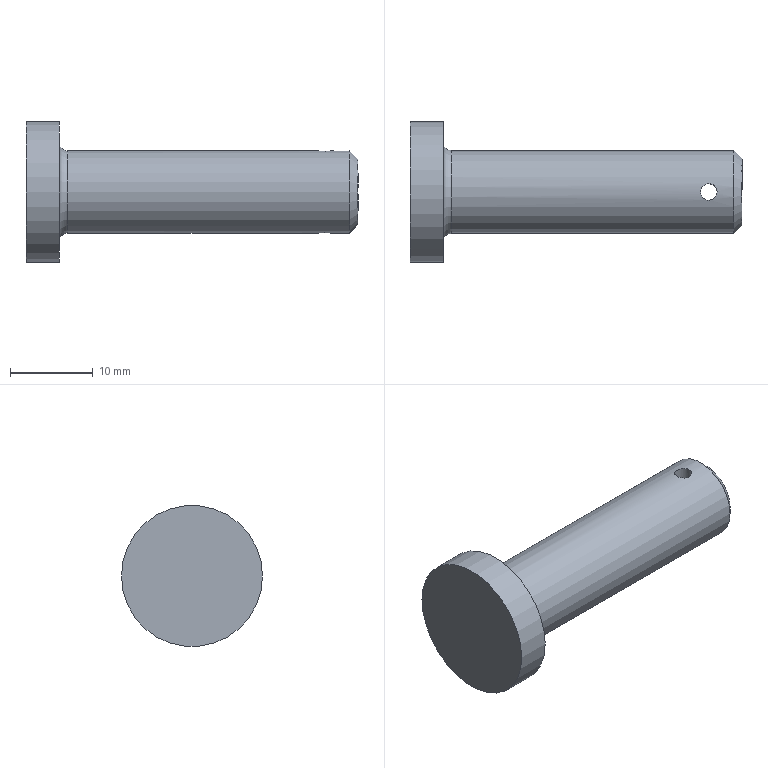Part | NX | features DATUM_CSYS 3, SKETCH 2, EXTRUDE 1, SWP104 1 | 1 solid | 8 faces | box 40 x 17 x 17 mm | volume 3696 mm3 | cylinder 3 | plane 3 | torus 1 | cone 1 | commonest cylinder face diameters 2 x1 10 x1 17 x1
STEP:
#1=CARTESIAN_POINT('',(39.,5.,0.));
#2=VERTEX_POINT('',#1);
#3=CARTESIAN_POINT('',(39.,0.,0.));
#4=DIRECTION('',(1.,0.,0.));
#5=DIRECTION('',(0.,1.,0.));
#6=AXIS2_PLACEMENT_3D('',#3,#4,#5);
#7=CIRCLE('',#6,5.);
#8=EDGE_CURVE('',#2,#2,#7,.T.);
#9=ORIENTED_EDGE('',*,*,#8,.F.);
#10=EDGE_LOOP('',(#9));
#11=FACE_BOUND('',#10,.T.);
#12=CARTESIAN_POINT('',(5.,5.,0.));
#13=VERTEX_POINT('',#12);
#14=CARTESIAN_POINT('',(5.,0.,0.));
#15=DIRECTION('',(1.,0.,0.));
#16=DIRECTION('',(0.,1.,0.));
#17=AXIS2_PLACEMENT_3D('',#14,#15,#16);
#18=CIRCLE('',#17,5.);
#19=EDGE_CURVE('',#13,#13,#18,.T.);
#20=ORIENTED_EDGE('',*,*,#19,.T.);
#21=EDGE_LOOP('',(#20));
#22=FACE_BOUND('',#21,.T.);
#23=CARTESIAN_POINT('',(35.,0.,-5.));
#24=VERTEX_POINT('',#23);
#25=CARTESIAN_POINT('',(35.217,-0.7844,-4.95));
#26=CARTESIAN_POINT('',(34.892,0.0001751,-5.025));
#27=CARTESIAN_POINT('',(35.217,0.7837,-4.95));
#28=CARTESIAN_POINT('',(35.999,1.108,-4.873));
#29=CARTESIAN_POINT('',(36.784,0.7838,-4.95));
#30=CARTESIAN_POINT('',(37.108,0.0003593,-5.025));
#31=CARTESIAN_POINT('',(36.784,-0.7828,-4.95));
#32=CARTESIAN_POINT('',(36.001,-1.108,-4.873));
#33=CARTESIAN_POINT('',(35.217,-0.7844,-4.95));
#34=CARTESIAN_POINT('',(34.892,0.0001751,-5.025));
#35=CARTESIAN_POINT('',(35.217,0.7837,-4.95));
#36=B_SPLINE_CURVE_WITH_KNOTS('',3,(#25,#26,#27,#28,#29,#30,#31,#32,#33,#34,#35),.UNSPECIFIED.,.T.,.F.,(1,1,1,1,1,1,1,1,1,1,1,1,1,1,1),(-0.00235,-0.001567,-0.0007835,0.,0.0007835,0.001567,0.00235,0.003134,0.003917,0.004701,0.005484,0.006268,0.007051,0.007835,0.008618),.UNSPECIFIED.);
#37=EDGE_CURVE('',#24,#24,#36,.T.);
#38=ORIENTED_EDGE('',*,*,#37,.F.);
#39=EDGE_LOOP('',(#38));
#40=FACE_BOUND('',#39,.T.);
#41=CARTESIAN_POINT('',(35.,0.,5.));
#42=VERTEX_POINT('',#41);
#43=CARTESIAN_POINT('',(35.217,0.7844,4.95));
#44=CARTESIAN_POINT('',(34.892,-0.0001751,5.025));
#45=CARTESIAN_POINT('',(35.217,-0.7837,4.95));
#46=CARTESIAN_POINT('',(35.999,-1.108,4.873));
#47=CARTESIAN_POINT('',(36.784,-0.7838,4.95));
#48=CARTESIAN_POINT('',(37.108,-0.0003593,5.025));
#49=CARTESIAN_POINT('',(36.784,0.7828,4.95));
#50=CARTESIAN_POINT('',(36.001,1.108,4.873));
#51=CARTESIAN_POINT('',(35.217,0.7844,4.95));
#52=CARTESIAN_POINT('',(34.892,-0.0001751,5.025));
#53=CARTESIAN_POINT('',(35.217,-0.7837,4.95));
#54=B_SPLINE_CURVE_WITH_KNOTS('',3,(#43,#44,#45,#46,#47,#48,#49,#50,#51,#52,#53),.UNSPECIFIED.,.T.,.F.,(1,1,1,1,1,1,1,1,1,1,1,1,1,1,1),(-0.00235,-0.001567,-0.0007835,0.,0.0007835,0.001567,0.00235,0.003134,0.003917,0.004701,0.005484,0.006268,0.007051,0.007835,0.008618),.UNSPECIFIED.);
#55=EDGE_CURVE('',#42,#42,#54,.T.);
#56=ORIENTED_EDGE('',*,*,#55,.F.);
#57=EDGE_LOOP('',(#56));
#58=FACE_BOUND('',#57,.T.);
#59=CARTESIAN_POINT('',(0.,0.,0.));
#60=DIRECTION('',(1.,0.,0.));
#61=DIRECTION('',(0.,1.,0.));
#62=AXIS2_PLACEMENT_3D('',#59,#60,#61);
#63=CYLINDRICAL_SURFACE('',#62,5.);
#64=ADVANCED_FACE('',(#11,#22,#40,#58),#63,.T.);
#65=CARTESIAN_POINT('',(0.,8.5,0.));
#66=VERTEX_POINT('',#65);
#67=CARTESIAN_POINT('',(0.,0.,0.));
#68=DIRECTION('',(1.,0.,0.));
#69=DIRECTION('',(0.,1.,0.));
#70=AXIS2_PLACEMENT_3D('',#67,#68,#69);
#71=CIRCLE('',#70,8.5);
#72=EDGE_CURVE('',#66,#66,#71,.T.);
#73=ORIENTED_EDGE('',*,*,#72,.F.);
#74=EDGE_LOOP('',(#73));
#75=FACE_BOUND('',#74,.T.);
#76=CARTESIAN_POINT('',(0.,0.,0.));
#77=DIRECTION('',(1.,0.,0.));
#78=DIRECTION('',(0.,1.,0.));
#79=AXIS2_PLACEMENT_3D('',#76,#77,#78);
#80=PLANE('',#79);
#81=ADVANCED_FACE('',(#75),#80,.F.);
#82=CARTESIAN_POINT('',(4.,8.5,0.));
#83=VERTEX_POINT('',#82);
#84=CARTESIAN_POINT('',(4.,0.,0.));
#85=DIRECTION('',(1.,0.,0.));
#86=DIRECTION('',(0.,1.,0.));
#87=AXIS2_PLACEMENT_3D('',#84,#85,#86);
#88=CIRCLE('',#87,8.5);
#89=EDGE_CURVE('',#83,#83,#88,.T.);
#90=ORIENTED_EDGE('',*,*,#89,.F.);
#91=EDGE_LOOP('',(#90));
#92=FACE_BOUND('',#91,.T.);
#93=ORIENTED_EDGE('',*,*,#72,.T.);
#94=EDGE_LOOP('',(#93));
#95=FACE_BOUND('',#94,.T.);
#96=CARTESIAN_POINT('',(0.,0.,0.));
#97=DIRECTION('',(1.,0.,0.));
#98=DIRECTION('',(0.,1.,0.));
#99=AXIS2_PLACEMENT_3D('',#96,#97,#98);
#100=CYLINDRICAL_SURFACE('',#99,8.5);
#101=ADVANCED_FACE('',(#92,#95),#100,.T.);
#102=CARTESIAN_POINT('',(4.,6.,0.));
#103=VERTEX_POINT('',#102);
#104=CARTESIAN_POINT('',(4.,0.,0.));
#105=DIRECTION('',(1.,0.,0.));
#106=DIRECTION('',(0.,1.,0.));
#107=AXIS2_PLACEMENT_3D('',#104,#105,#106);
#108=CIRCLE('',#107,6.);
#109=EDGE_CURVE('',#103,#103,#108,.T.);
#110=ORIENTED_EDGE('',*,*,#109,.F.);
#111=EDGE_LOOP('',(#110));
#112=FACE_BOUND('',#111,.T.);
#113=ORIENTED_EDGE('',*,*,#89,.T.);
#114=EDGE_LOOP('',(#113));
#115=FACE_BOUND('',#114,.T.);
#116=CARTESIAN_POINT('',(4.,8.5,0.));
#117=DIRECTION('',(-1.,0.,0.));
#118=DIRECTION('',(0.,-1.,0.));
#119=AXIS2_PLACEMENT_3D('',#116,#117,#118);
#120=PLANE('',#119);
#121=ADVANCED_FACE('',(#112,#115),#120,.F.);
#122=ORIENTED_EDGE('',*,*,#19,.F.);
#123=EDGE_LOOP('',(#122));
#124=FACE_BOUND('',#123,.T.);
#125=ORIENTED_EDGE('',*,*,#109,.T.);
#126=EDGE_LOOP('',(#125));
#127=FACE_BOUND('',#126,.T.);
#128=CARTESIAN_POINT('',(5.,0.,0.));
#129=DIRECTION('',(1.,0.,0.));
#130=DIRECTION('',(0.,1.,0.));
#131=AXIS2_PLACEMENT_3D('',#128,#129,#130);
#132=TOROIDAL_SURFACE('',#131,6.,1.);
#133=ADVANCED_FACE('',(#124,#127),#132,.F.);
#134=CARTESIAN_POINT('',(40.,4.,0.));
#135=VERTEX_POINT('',#134);
#136=CARTESIAN_POINT('',(40.,0.,0.));
#137=DIRECTION('',(1.,0.,0.));
#138=DIRECTION('',(0.,1.,0.));
#139=AXIS2_PLACEMENT_3D('',#136,#137,#138);
#140=CIRCLE('',#139,4.);
#141=EDGE_CURVE('',#135,#135,#140,.T.);
#142=ORIENTED_EDGE('',*,*,#141,.F.);
#143=EDGE_LOOP('',(#142));
#144=FACE_BOUND('',#143,.T.);
#145=ORIENTED_EDGE('',*,*,#8,.T.);
#146=EDGE_LOOP('',(#145));
#147=FACE_BOUND('',#146,.T.);
#148=CARTESIAN_POINT('',(39.,0.,0.));
#149=DIRECTION('',(-1.,0.,0.));
#150=DIRECTION('',(0.,-1.,0.));
#151=AXIS2_PLACEMENT_3D('',#148,#149,#150);
#152=CONICAL_SURFACE('',#151,5.,0.7854);
#153=ADVANCED_FACE('',(#144,#147),#152,.T.);
#154=ORIENTED_EDGE('',*,*,#141,.T.);
#155=EDGE_LOOP('',(#154));
#156=FACE_BOUND('',#155,.T.);
#157=CARTESIAN_POINT('',(40.,4.,0.));
#158=DIRECTION('',(-1.,0.,0.));
#159=DIRECTION('',(0.,-1.,0.));
#160=AXIS2_PLACEMENT_3D('',#157,#158,#159);
#161=PLANE('',#160);
#162=ADVANCED_FACE('',(#156),#161,.F.);
#163=ORIENTED_EDGE('',*,*,#37,.T.);
#164=EDGE_LOOP('',(#163));
#165=FACE_BOUND('',#164,.T.);
#166=ORIENTED_EDGE('',*,*,#55,.T.);
#167=EDGE_LOOP('',(#166));
#168=FACE_BOUND('',#167,.T.);
#169=CARTESIAN_POINT('',(36.,0.,16.9));
#170=DIRECTION('',(0.,0.,-1.));
#171=DIRECTION('',(-1.,0.,0.));
#172=AXIS2_PLACEMENT_3D('',#169,#170,#171);
#173=CYLINDRICAL_SURFACE('',#172,1.);
#174=ADVANCED_FACE('',(#165,#168),#173,.F.);
#175=CLOSED_SHELL('',(#64,#81,#101,#121,#133,#153,#162,#174));
#176=MANIFOLD_SOLID_BREP('',#175);
#177=(LENGTH_UNIT()NAMED_UNIT(*)SI_UNIT(.MILLI.,.METRE.));
#178=UNCERTAINTY_MEASURE_WITH_UNIT(LENGTH_MEASURE(0.0508),#177,'','');
#179=(NAMED_UNIT(*)PLANE_ANGLE_UNIT()SI_UNIT($,.RADIAN.));
#180=(NAMED_UNIT(*)SI_UNIT($,.STERADIAN.)SOLID_ANGLE_UNIT());
#181=(GEOMETRIC_REPRESENTATION_CONTEXT(3)GLOBAL_UNCERTAINTY_ASSIGNED_CONTEXT((#178))GLOBAL_UNIT_ASSIGNED_CONTEXT((#177,#179,#180))REPRESENTATION_CONTEXT('',''));
#182=ADVANCED_BREP_SHAPE_REPRESENTATION('',(#176),#181);